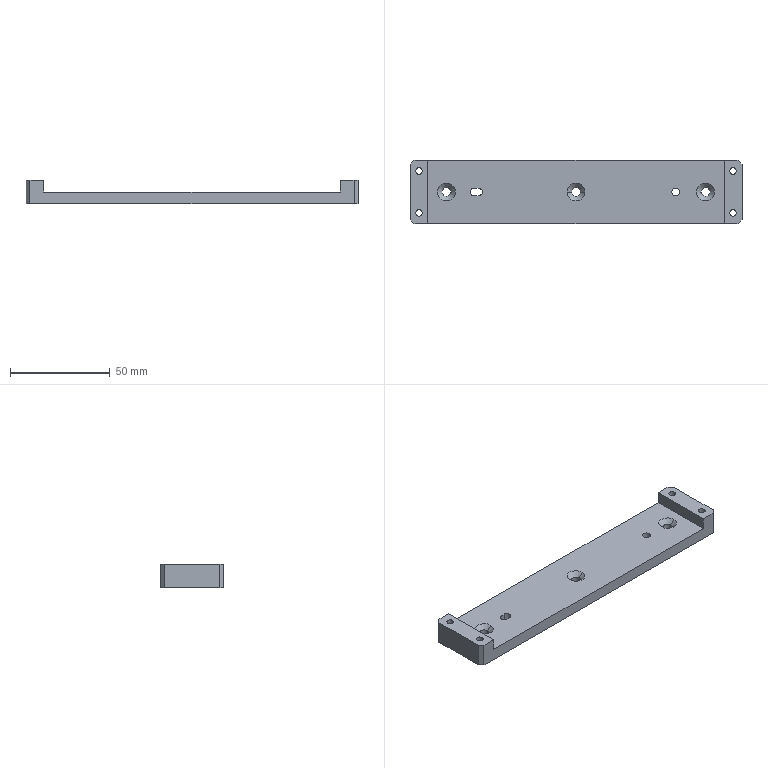Part | STEP file | QA-AD06 | 1 solid | 41 faces | box 166.5 x 32 x 12 mm | volume 34292 mm3 | cylinder 19 | plane 16 | cone 6 | commonest cylinder face diameters 3.3 x8 4.5 x6 4 x5